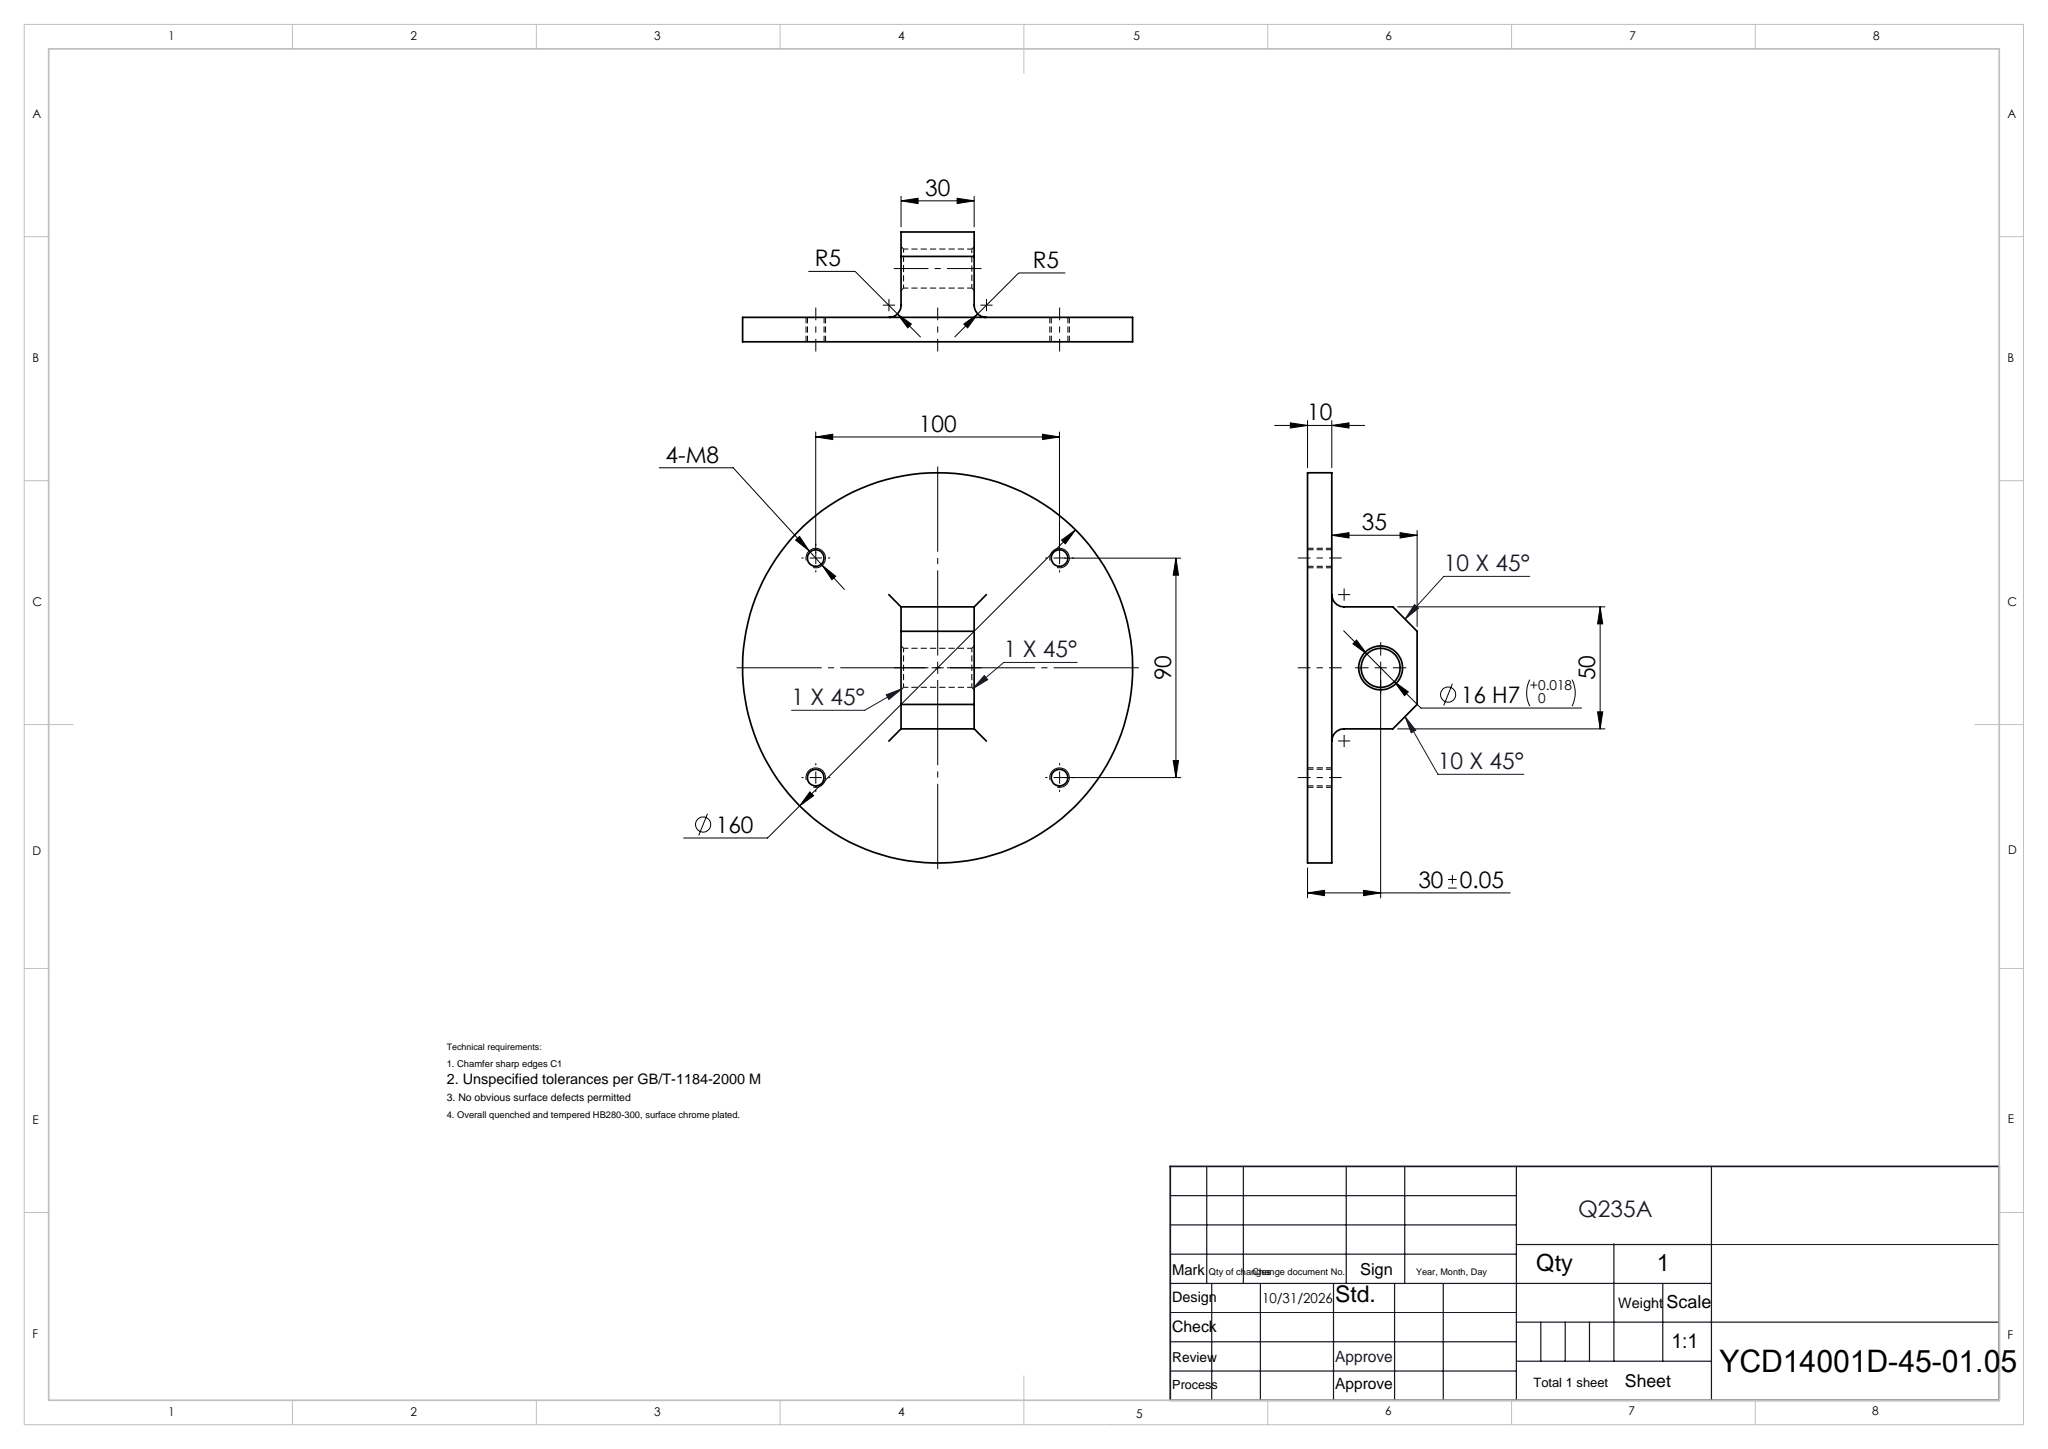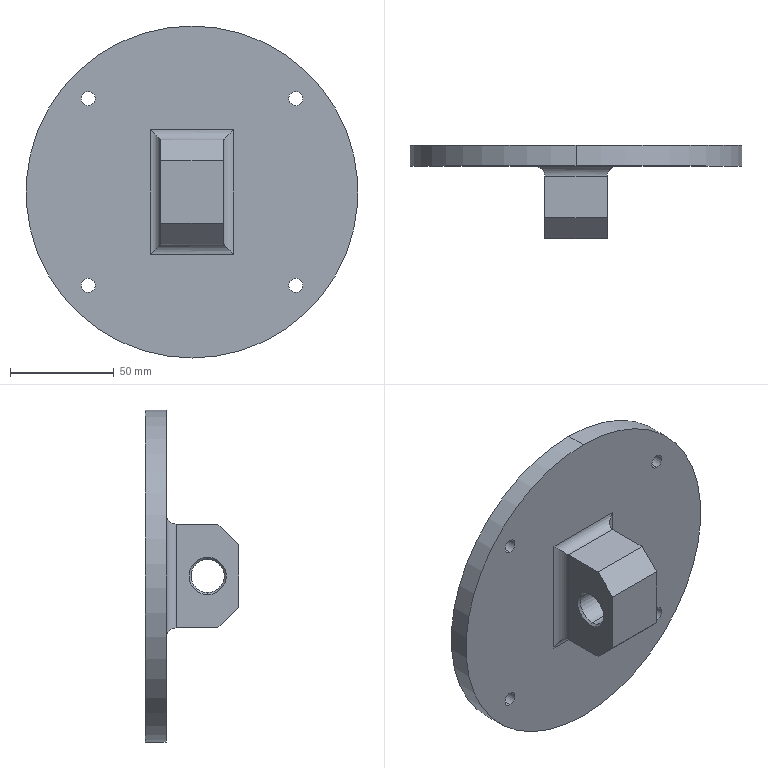Part | SolidWorks | features ICE 3, Chamfer 2, Fillet 2, Extrusion 1, HoleWzd 1 | 1 solid | 29 faces | box 160 x 45 x 160 mm | volume 243931 mm3 | cylinder 16 | plane 9 | cone 4 | commonest cylinder face diameters 6.8 x8 10 x4 16 x2 160 x2
STEP:
#1=CARTESIAN_POINT('',(14.,-25.,8.));
#2=VERTEX_POINT('',#1);
#3=CARTESIAN_POINT('',(14.,-25.,-8.));
#4=VERTEX_POINT('',#3);
#5=CARTESIAN_POINT('',(14.,-25.,0.));
#6=DIRECTION('',(1.,0.,0.));
#7=DIRECTION('',(0.,0.,1.));
#8=AXIS2_PLACEMENT_3D('',#5,#6,#7);
#9=CIRCLE('',#8,8.);
#10=EDGE_CURVE('',#2,#4,#9,.T.);
#11=ORIENTED_EDGE('',*,*,#10,.F.);
#12=CARTESIAN_POINT('',(15.,-25.,9.));
#13=VERTEX_POINT('',#12);
#14=CARTESIAN_POINT('',(14.,-25.,8.));
#15=DIRECTION('',(0.7071,0.,0.7071));
#16=VECTOR('',#15,1000.);
#17=LINE('',#14,#16);
#18=EDGE_CURVE('',#2,#13,#17,.T.);
#19=ORIENTED_EDGE('',*,*,#18,.T.);
#20=CARTESIAN_POINT('',(15.,-25.,-9.));
#21=VERTEX_POINT('',#20);
#22=CARTESIAN_POINT('',(15.,-25.,0.));
#23=DIRECTION('',(-1.,0.,0.));
#24=DIRECTION('',(0.,0.,1.));
#25=AXIS2_PLACEMENT_3D('',#22,#23,#24);
#26=CIRCLE('',#25,9.);
#27=EDGE_CURVE('',#21,#13,#26,.T.);
#28=ORIENTED_EDGE('',*,*,#27,.F.);
#29=CARTESIAN_POINT('',(14.,-25.,-8.));
#30=DIRECTION('',(0.7071,0.,-0.7071));
#31=VECTOR('',#30,1000.);
#32=LINE('',#29,#31);
#33=EDGE_CURVE('',#4,#21,#32,.T.);
#34=ORIENTED_EDGE('',*,*,#33,.F.);
#35=EDGE_LOOP('',(#11,#19,#28,#34));
#36=FACE_OUTER_BOUND('',#35,.T.);
#37=CARTESIAN_POINT('',(14.,-25.,0.));
#38=DIRECTION('',(1.,0.,0.));
#39=DIRECTION('',(0.,0.,-1.));
#40=AXIS2_PLACEMENT_3D('',#37,#38,#39);
#41=CONICAL_SURFACE('',#40,8.,0.7854);
#42=ADVANCED_FACE('',(#36),#41,.F.);
#43=CARTESIAN_POINT('',(-14.,-25.,-8.));
#44=VERTEX_POINT('',#43);
#45=CARTESIAN_POINT('',(-14.,-25.,8.));
#46=VERTEX_POINT('',#45);
#47=CARTESIAN_POINT('',(-14.,-25.,0.));
#48=DIRECTION('',(-1.,0.,0.));
#49=DIRECTION('',(0.,0.,-1.));
#50=AXIS2_PLACEMENT_3D('',#47,#48,#49);
#51=CIRCLE('',#50,8.);
#52=EDGE_CURVE('',#44,#46,#51,.T.);
#53=ORIENTED_EDGE('',*,*,#52,.F.);
#54=CARTESIAN_POINT('',(-15.,-25.,-9.));
#55=VERTEX_POINT('',#54);
#56=CARTESIAN_POINT('',(-15.,-25.,-9.));
#57=DIRECTION('',(-0.7071,0.,-0.7071));
#58=VECTOR('',#57,1000.);
#59=LINE('',#56,#58);
#60=EDGE_CURVE('',#44,#55,#59,.T.);
#61=ORIENTED_EDGE('',*,*,#60,.T.);
#62=CARTESIAN_POINT('',(-15.,-25.,9.));
#63=VERTEX_POINT('',#62);
#64=CARTESIAN_POINT('',(-15.,-25.,0.));
#65=DIRECTION('',(1.,0.,0.));
#66=DIRECTION('',(0.,0.,-1.));
#67=AXIS2_PLACEMENT_3D('',#64,#65,#66);
#68=CIRCLE('',#67,9.);
#69=EDGE_CURVE('',#63,#55,#68,.T.);
#70=ORIENTED_EDGE('',*,*,#69,.F.);
#71=CARTESIAN_POINT('',(-15.,-25.,9.));
#72=DIRECTION('',(-0.7071,0.,0.7071));
#73=VECTOR('',#72,1000.);
#74=LINE('',#71,#73);
#75=EDGE_CURVE('',#46,#63,#74,.T.);
#76=ORIENTED_EDGE('',*,*,#75,.F.);
#77=EDGE_LOOP('',(#53,#61,#70,#76));
#78=FACE_OUTER_BOUND('',#77,.T.);
#79=CARTESIAN_POINT('',(-15.,-25.,0.));
#80=DIRECTION('',(-1.,0.,0.));
#81=DIRECTION('',(0.,0.,1.));
#82=AXIS2_PLACEMENT_3D('',#79,#80,#81);
#83=CONICAL_SURFACE('',#82,9.,0.7854);
#84=ADVANCED_FACE('',(#78),#83,.F.);
#85=ORIENTED_EDGE('',*,*,#52,.T.);
#86=CARTESIAN_POINT('',(-80.,-25.,8.));
#87=DIRECTION('',(1.,0.,0.));
#88=VECTOR('',#87,1000.);
#89=LINE('',#86,#88);
#90=EDGE_CURVE('',#46,#2,#89,.T.);
#91=ORIENTED_EDGE('',*,*,#90,.T.);
#92=ORIENTED_EDGE('',*,*,#10,.T.);
#93=CARTESIAN_POINT('',(-80.,-25.,-8.));
#94=DIRECTION('',(1.,0.,0.));
#95=VECTOR('',#94,1000.);
#96=LINE('',#93,#95);
#97=EDGE_CURVE('',#44,#4,#96,.T.);
#98=ORIENTED_EDGE('',*,*,#97,.F.);
#99=EDGE_LOOP('',(#85,#91,#92,#98));
#100=FACE_OUTER_BOUND('',#99,.T.);
#101=CARTESIAN_POINT('',(-80.,-25.,0.));
#102=DIRECTION('',(1.,0.,0.));
#103=DIRECTION('',(0.,0.,-1.));
#104=AXIS2_PLACEMENT_3D('',#101,#102,#103);
#105=CYLINDRICAL_SURFACE('',#104,8.);
#106=ADVANCED_FACE('',(#100),#105,.F.);
#107=CARTESIAN_POINT('',(-50.,5.,48.4));
#108=VERTEX_POINT('',#107);
#109=CARTESIAN_POINT('',(-50.,5.,41.6));
#110=VERTEX_POINT('',#109);
#111=CARTESIAN_POINT('',(-50.,5.,45.));
#112=DIRECTION('',(0.,-1.,0.));
#113=DIRECTION('',(0.,0.,-1.));
#114=AXIS2_PLACEMENT_3D('',#111,#112,#113);
#115=CIRCLE('',#114,3.4);
#116=EDGE_CURVE('',#108,#110,#115,.T.);
#117=ORIENTED_EDGE('',*,*,#116,.F.);
#118=CARTESIAN_POINT('',(-50.,-5.,48.4));
#119=VERTEX_POINT('',#118);
#120=CARTESIAN_POINT('',(-50.,-5.,48.4));
#121=DIRECTION('',(0.,-1.,0.));
#122=VECTOR('',#121,1000.);
#123=LINE('',#120,#122);
#124=EDGE_CURVE('',#108,#119,#123,.T.);
#125=ORIENTED_EDGE('',*,*,#124,.T.);
#126=CARTESIAN_POINT('',(-50.,-5.,41.6));
#127=VERTEX_POINT('',#126);
#128=CARTESIAN_POINT('',(-50.,-5.,45.));
#129=DIRECTION('',(0.,-1.,0.));
#130=DIRECTION('',(0.,0.,-1.));
#131=AXIS2_PLACEMENT_3D('',#128,#129,#130);
#132=CIRCLE('',#131,3.4);
#133=EDGE_CURVE('',#119,#127,#132,.T.);
#134=ORIENTED_EDGE('',*,*,#133,.T.);
#135=CARTESIAN_POINT('',(-50.,-5.,41.6));
#136=DIRECTION('',(0.,-1.,0.));
#137=VECTOR('',#136,1000.);
#138=LINE('',#135,#137);
#139=EDGE_CURVE('',#110,#127,#138,.T.);
#140=ORIENTED_EDGE('',*,*,#139,.F.);
#141=EDGE_LOOP('',(#117,#125,#134,#140));
#142=FACE_OUTER_BOUND('',#141,.T.);
#143=CARTESIAN_POINT('',(-50.,-5.,45.));
#144=DIRECTION('',(0.,-1.,0.));
#145=DIRECTION('',(0.,0.,-1.));
#146=AXIS2_PLACEMENT_3D('',#143,#144,#145);
#147=CYLINDRICAL_SURFACE('',#146,3.4);
#148=ADVANCED_FACE('',(#142),#147,.F.);
#149=CARTESIAN_POINT('',(-50.,5.,-41.6));
#150=VERTEX_POINT('',#149);
#151=CARTESIAN_POINT('',(-50.,5.,-48.4));
#152=VERTEX_POINT('',#151);
#153=CARTESIAN_POINT('',(-50.,5.,-45.));
#154=DIRECTION('',(0.,-1.,0.));
#155=DIRECTION('',(0.,0.,-1.));
#156=AXIS2_PLACEMENT_3D('',#153,#154,#155);
#157=CIRCLE('',#156,3.4);
#158=EDGE_CURVE('',#150,#152,#157,.T.);
#159=ORIENTED_EDGE('',*,*,#158,.F.);
#160=CARTESIAN_POINT('',(-50.,-5.,-41.6));
#161=VERTEX_POINT('',#160);
#162=CARTESIAN_POINT('',(-50.,-5.,-41.6));
#163=DIRECTION('',(0.,-1.,0.));
#164=VECTOR('',#163,1000.);
#165=LINE('',#162,#164);
#166=EDGE_CURVE('',#150,#161,#165,.T.);
#167=ORIENTED_EDGE('',*,*,#166,.T.);
#168=CARTESIAN_POINT('',(-50.,-5.,-48.4));
#169=VERTEX_POINT('',#168);
#170=CARTESIAN_POINT('',(-50.,-5.,-45.));
#171=DIRECTION('',(0.,-1.,0.));
#172=DIRECTION('',(0.,0.,-1.));
#173=AXIS2_PLACEMENT_3D('',#170,#171,#172);
#174=CIRCLE('',#173,3.4);
#175=EDGE_CURVE('',#161,#169,#174,.T.);
#176=ORIENTED_EDGE('',*,*,#175,.T.);
#177=CARTESIAN_POINT('',(-50.,-5.,-48.4));
#178=DIRECTION('',(0.,-1.,0.));
#179=VECTOR('',#178,1000.);
#180=LINE('',#177,#179);
#181=EDGE_CURVE('',#152,#169,#180,.T.);
#182=ORIENTED_EDGE('',*,*,#181,.F.);
#183=EDGE_LOOP('',(#159,#167,#176,#182));
#184=FACE_OUTER_BOUND('',#183,.T.);
#185=CARTESIAN_POINT('',(-50.,-5.,-45.));
#186=DIRECTION('',(0.,-1.,0.));
#187=DIRECTION('',(0.,0.,-1.));
#188=AXIS2_PLACEMENT_3D('',#185,#186,#187);
#189=CYLINDRICAL_SURFACE('',#188,3.4);
#190=ADVANCED_FACE('',(#184),#189,.F.);
#191=CARTESIAN_POINT('',(50.,5.,-41.6));
#192=VERTEX_POINT('',#191);
#193=CARTESIAN_POINT('',(50.,5.,-48.4));
#194=VERTEX_POINT('',#193);
#195=CARTESIAN_POINT('',(50.,5.,-45.));
#196=DIRECTION('',(0.,-1.,0.));
#197=DIRECTION('',(0.,0.,-1.));
#198=AXIS2_PLACEMENT_3D('',#195,#196,#197);
#199=CIRCLE('',#198,3.4);
#200=EDGE_CURVE('',#192,#194,#199,.T.);
#201=ORIENTED_EDGE('',*,*,#200,.F.);
#202=CARTESIAN_POINT('',(50.,-5.,-41.6));
#203=VERTEX_POINT('',#202);
#204=CARTESIAN_POINT('',(50.,-5.,-41.6));
#205=DIRECTION('',(0.,-1.,0.));
#206=VECTOR('',#205,1000.);
#207=LINE('',#204,#206);
#208=EDGE_CURVE('',#192,#203,#207,.T.);
#209=ORIENTED_EDGE('',*,*,#208,.T.);
#210=CARTESIAN_POINT('',(50.,-5.,-48.4));
#211=VERTEX_POINT('',#210);
#212=CARTESIAN_POINT('',(50.,-5.,-45.));
#213=DIRECTION('',(0.,-1.,0.));
#214=DIRECTION('',(0.,0.,-1.));
#215=AXIS2_PLACEMENT_3D('',#212,#213,#214);
#216=CIRCLE('',#215,3.4);
#217=EDGE_CURVE('',#203,#211,#216,.T.);
#218=ORIENTED_EDGE('',*,*,#217,.T.);
#219=CARTESIAN_POINT('',(50.,-5.,-48.4));
#220=DIRECTION('',(0.,-1.,0.));
#221=VECTOR('',#220,1000.);
#222=LINE('',#219,#221);
#223=EDGE_CURVE('',#194,#211,#222,.T.);
#224=ORIENTED_EDGE('',*,*,#223,.F.);
#225=EDGE_LOOP('',(#201,#209,#218,#224));
#226=FACE_OUTER_BOUND('',#225,.T.);
#227=CARTESIAN_POINT('',(50.,-5.,-45.));
#228=DIRECTION('',(0.,-1.,0.));
#229=DIRECTION('',(0.,0.,-1.));
#230=AXIS2_PLACEMENT_3D('',#227,#228,#229);
#231=CYLINDRICAL_SURFACE('',#230,3.4);
#232=ADVANCED_FACE('',(#226),#231,.F.);
#233=CARTESIAN_POINT('',(50.,5.,48.4));
#234=VERTEX_POINT('',#233);
#235=CARTESIAN_POINT('',(50.,5.,41.6));
#236=VERTEX_POINT('',#235);
#237=CARTESIAN_POINT('',(50.,5.,45.));
#238=DIRECTION('',(0.,-1.,0.));
#239=DIRECTION('',(0.,0.,-1.));
#240=AXIS2_PLACEMENT_3D('',#237,#238,#239);
#241=CIRCLE('',#240,3.4);
#242=EDGE_CURVE('',#234,#236,#241,.T.);
#243=ORIENTED_EDGE('',*,*,#242,.F.);
#244=CARTESIAN_POINT('',(50.,-5.,48.4));
#245=VERTEX_POINT('',#244);
#246=CARTESIAN_POINT('',(50.,-5.,48.4));
#247=DIRECTION('',(0.,-1.,0.));
#248=VECTOR('',#247,1000.);
#249=LINE('',#246,#248);
#250=EDGE_CURVE('',#234,#245,#249,.T.);
#251=ORIENTED_EDGE('',*,*,#250,.T.);
#252=CARTESIAN_POINT('',(50.,-5.,41.6));
#253=VERTEX_POINT('',#252);
#254=CARTESIAN_POINT('',(50.,-5.,45.));
#255=DIRECTION('',(0.,-1.,0.));
#256=DIRECTION('',(0.,0.,-1.));
#257=AXIS2_PLACEMENT_3D('',#254,#255,#256);
#258=CIRCLE('',#257,3.4);
#259=EDGE_CURVE('',#245,#253,#258,.T.);
#260=ORIENTED_EDGE('',*,*,#259,.T.);
#261=CARTESIAN_POINT('',(50.,-5.,41.6));
#262=DIRECTION('',(0.,-1.,0.));
#263=VECTOR('',#262,1000.);
#264=LINE('',#261,#263);
#265=EDGE_CURVE('',#236,#253,#264,.T.);
#266=ORIENTED_EDGE('',*,*,#265,.F.);
#267=EDGE_LOOP('',(#243,#251,#260,#266));
#268=FACE_OUTER_BOUND('',#267,.T.);
#269=CARTESIAN_POINT('',(50.,-5.,45.));
#270=DIRECTION('',(0.,-1.,0.));
#271=DIRECTION('',(0.,0.,-1.));
#272=AXIS2_PLACEMENT_3D('',#269,#270,#271);
#273=CYLINDRICAL_SURFACE('',#272,3.4);
#274=ADVANCED_FACE('',(#268),#273,.F.);
#275=CARTESIAN_POINT('',(0.,5.,80.));
#276=VERTEX_POINT('',#275);
#277=CARTESIAN_POINT('',(0.,5.,-80.));
#278=VERTEX_POINT('',#277);
#279=CARTESIAN_POINT('',(0.,5.,0.));
#280=DIRECTION('',(0.,1.,0.));
#281=DIRECTION('',(0.,0.,1.));
#282=AXIS2_PLACEMENT_3D('',#279,#280,#281);
#283=CIRCLE('',#282,80.);
#284=EDGE_CURVE('',#276,#278,#283,.T.);
#285=ORIENTED_EDGE('',*,*,#284,.F.);
#286=CARTESIAN_POINT('',(0.,-5.,80.));
#287=VERTEX_POINT('',#286);
#288=CARTESIAN_POINT('',(0.,5.,80.));
#289=DIRECTION('',(0.,-1.,0.));
#290=VECTOR('',#289,1000.);
#291=LINE('',#288,#290);
#292=EDGE_CURVE('',#276,#287,#291,.T.);
#293=ORIENTED_EDGE('',*,*,#292,.T.);
#294=CARTESIAN_POINT('',(0.,-5.,-80.));
#295=VERTEX_POINT('',#294);
#296=CARTESIAN_POINT('',(0.,-5.,0.));
#297=DIRECTION('',(0.,1.,0.));
#298=DIRECTION('',(0.,0.,1.));
#299=AXIS2_PLACEMENT_3D('',#296,#297,#298);
#300=CIRCLE('',#299,80.);
#301=EDGE_CURVE('',#287,#295,#300,.T.);
#302=ORIENTED_EDGE('',*,*,#301,.T.);
#303=CARTESIAN_POINT('',(0.,5.,-80.));
#304=DIRECTION('',(0.,-1.,0.));
#305=VECTOR('',#304,1000.);
#306=LINE('',#303,#305);
#307=EDGE_CURVE('',#278,#295,#306,.T.);
#308=ORIENTED_EDGE('',*,*,#307,.F.);
#309=EDGE_LOOP('',(#285,#293,#302,#308));
#310=FACE_OUTER_BOUND('',#309,.T.);
#311=CARTESIAN_POINT('',(0.,5.,0.));
#312=DIRECTION('',(0.,-1.,0.));
#313=DIRECTION('',(0.,0.,-1.));
#314=AXIS2_PLACEMENT_3D('',#311,#312,#313);
#315=CYLINDRICAL_SURFACE('',#314,80.);
#316=ADVANCED_FACE('',(#310),#315,.T.);
#317=CARTESIAN_POINT('',(20.,-5.,30.));
#318=VERTEX_POINT('',#317);
#319=CARTESIAN_POINT('',(20.,-5.,-30.));
#320=VERTEX_POINT('',#319);
#321=CARTESIAN_POINT('',(20.,-5.,-25.));
#322=DIRECTION('',(0.,0.,-1.));
#323=VECTOR('',#322,1000.);
#324=LINE('',#321,#323);
#325=EDGE_CURVE('',#318,#320,#324,.T.);
#326=ORIENTED_EDGE('',*,*,#325,.T.);
#327=CARTESIAN_POINT('',(-20.,-5.,-30.));
#328=VERTEX_POINT('',#327);
#329=CARTESIAN_POINT('',(-15.,-5.,-30.));
#330=DIRECTION('',(-1.,0.,0.));
#331=VECTOR('',#330,1000.);
#332=LINE('',#329,#331);
#333=EDGE_CURVE('',#320,#328,#332,.T.);
#334=ORIENTED_EDGE('',*,*,#333,.T.);
#335=CARTESIAN_POINT('',(-20.,-5.,30.));
#336=VERTEX_POINT('',#335);
#337=CARTESIAN_POINT('',(-20.,-5.,25.));
#338=DIRECTION('',(0.,0.,1.));
#339=VECTOR('',#338,1000.);
#340=LINE('',#337,#339);
#341=EDGE_CURVE('',#328,#336,#340,.T.);
#342=ORIENTED_EDGE('',*,*,#341,.T.);
#343=CARTESIAN_POINT('',(15.,-5.,30.));
#344=DIRECTION('',(1.,0.,0.));
#345=VECTOR('',#344,1000.);
#346=LINE('',#343,#345);
#347=EDGE_CURVE('',#336,#318,#346,.T.);
#348=ORIENTED_EDGE('',*,*,#347,.T.);
#349=EDGE_LOOP('',(#326,#334,#342,#348));
#350=FACE_BOUND('',#349,.T.);
#351=CARTESIAN_POINT('',(0.,-5.,0.));
#352=DIRECTION('',(0.,1.,0.));
#353=DIRECTION('',(0.,0.,1.));
#354=AXIS2_PLACEMENT_3D('',#351,#352,#353);
#355=CIRCLE('',#354,80.);
#356=EDGE_CURVE('',#295,#287,#355,.T.);
#357=ORIENTED_EDGE('',*,*,#356,.F.);
#358=ORIENTED_EDGE('',*,*,#301,.F.);
#359=EDGE_LOOP('',(#357,#358));
#360=FACE_OUTER_BOUND('',#359,.T.);
#361=CARTESIAN_POINT('',(50.,-5.,45.));
#362=DIRECTION('',(0.,-1.,0.));
#363=DIRECTION('',(0.,0.,-1.));
#364=AXIS2_PLACEMENT_3D('',#361,#362,#363);
#365=CIRCLE('',#364,3.4);
#366=EDGE_CURVE('',#253,#245,#365,.T.);
#367=ORIENTED_EDGE('',*,*,#366,.F.);
#368=ORIENTED_EDGE('',*,*,#259,.F.);
#369=EDGE_LOOP('',(#367,#368));
#370=FACE_BOUND('',#369,.T.);
#371=CARTESIAN_POINT('',(50.,-5.,-45.));
#372=DIRECTION('',(0.,-1.,0.));
#373=DIRECTION('',(0.,0.,-1.));
#374=AXIS2_PLACEMENT_3D('',#371,#372,#373);
#375=CIRCLE('',#374,3.4);
#376=EDGE_CURVE('',#211,#203,#375,.T.);
#377=ORIENTED_EDGE('',*,*,#376,.F.);
#378=ORIENTED_EDGE('',*,*,#217,.F.);
#379=EDGE_LOOP('',(#377,#378));
#380=FACE_BOUND('',#379,.T.);
#381=CARTESIAN_POINT('',(-50.,-5.,-45.));
#382=DIRECTION('',(0.,-1.,0.));
#383=DIRECTION('',(0.,0.,-1.));
#384=AXIS2_PLACEMENT_3D('',#381,#382,#383);
#385=CIRCLE('',#384,3.4);
#386=EDGE_CURVE('',#169,#161,#385,.T.);
#387=ORIENTED_EDGE('',*,*,#386,.F.);
#388=ORIENTED_EDGE('',*,*,#175,.F.);
#389=EDGE_LOOP('',(#387,#388));
#390=FACE_BOUND('',#389,.T.);
#391=CARTESIAN_POINT('',(-50.,-5.,45.));
#392=DIRECTION('',(0.,-1.,0.));
#393=DIRECTION('',(0.,0.,-1.));
#394=AXIS2_PLACEMENT_3D('',#391,#392,#393);
#395=CIRCLE('',#394,3.4);
#396=EDGE_CURVE('',#127,#119,#395,.T.);
#397=ORIENTED_EDGE('',*,*,#396,.F.);
#398=ORIENTED_EDGE('',*,*,#133,.F.);
#399=EDGE_LOOP('',(#397,#398));
#400=FACE_BOUND('',#399,.T.);
#401=CARTESIAN_POINT('',(0.,-5.,0.));
#402=DIRECTION('',(0.,1.,0.));
#403=DIRECTION('',(0.,0.,1.));
#404=AXIS2_PLACEMENT_3D('',#401,#402,#403);
#405=PLANE('',#404);
#406=ADVANCED_FACE('',(#350,#360,#370,#380,#390,#400),#405,.F.);
#407=ORIENTED_EDGE('',*,*,#292,.F.);
#408=CARTESIAN_POINT('',(0.,5.,0.));
#409=DIRECTION('',(0.,1.,0.));
#410=DIRECTION('',(0.,0.,1.));
#411=AXIS2_PLACEMENT_3D('',#408,#409,#410);
#412=CIRCLE('',#411,80.);
#413=EDGE_CURVE('',#278,#276,#412,.T.);
#414=ORIENTED_EDGE('',*,*,#413,.F.);
#415=ORIENTED_EDGE('',*,*,#307,.T.);
#416=ORIENTED_EDGE('',*,*,#356,.T.);
#417=EDGE_LOOP('',(#407,#414,#415,#416));
#418=FACE_OUTER_BOUND('',#417,.T.);
#419=CARTESIAN_POINT('',(0.,5.,0.));
#420=DIRECTION('',(0.,-1.,0.));
#421=DIRECTION('',(0.,0.,-1.));
#422=AXIS2_PLACEMENT_3D('',#419,#420,#421);
#423=CYLINDRICAL_SURFACE('',#422,80.);
#424=ADVANCED_FACE('',(#418),#423,.T.);
#425=CARTESIAN_POINT('',(-50.,5.,45.));
#426=DIRECTION('',(0.,-1.,0.));
#427=DIRECTION('',(0.,0.,-1.));
#428=AXIS2_PLACEMENT_3D('',#425,#426,#427);
#429=CIRCLE('',#428,3.4);
#430=EDGE_CURVE('',#110,#108,#429,.T.);
#431=ORIENTED_EDGE('',*,*,#430,.T.);
#432=ORIENTED_EDGE('',*,*,#116,.T.);
#433=EDGE_LOOP('',(#431,#432));
#434=FACE_BOUND('',#433,.T.);
#435=CARTESIAN_POINT('',(-50.,5.,-45.));
#436=DIRECTION('',(0.,-1.,0.));
#437=DIRECTION('',(0.,0.,-1.));
#438=AXIS2_PLACEMENT_3D('',#435,#436,#437);
#439=CIRCLE('',#438,3.4);
#440=EDGE_CURVE('',#152,#150,#439,.T.);
#441=ORIENTED_EDGE('',*,*,#440,.T.);
#442=ORIENTED_EDGE('',*,*,#158,.T.);
#443=EDGE_LOOP('',(#441,#442));
#444=FACE_BOUND('',#443,.T.);
#445=CARTESIAN_POINT('',(50.,5.,-45.));
#446=DIRECTION('',(0.,-1.,0.));
#447=DIRECTION('',(0.,0.,-1.));
#448=AXIS2_PLACEMENT_3D('',#445,#446,#447);
#449=CIRCLE('',#448,3.4);
#450=EDGE_CURVE('',#194,#192,#449,.T.);
#451=ORIENTED_EDGE('',*,*,#450,.T.);
#452=ORIENTED_EDGE('',*,*,#200,.T.);
#453=EDGE_LOOP('',(#451,#452));
#454=FACE_BOUND('',#453,.T.);
#455=CARTESIAN_POINT('',(50.,5.,45.));
#456=DIRECTION('',(0.,-1.,0.));
#457=DIRECTION('',(0.,0.,-1.));
#458=AXIS2_PLACEMENT_3D('',#455,#456,#457);
#459=CIRCLE('',#458,3.4);
#460=EDGE_CURVE('',#236,#234,#459,.T.);
#461=ORIENTED_EDGE('',*,*,#460,.T.);
#462=ORIENTED_EDGE('',*,*,#242,.T.);
#463=EDGE_LOOP('',(#461,#462));
#464=FACE_BOUND('',#463,.T.);
#465=ORIENTED_EDGE('',*,*,#413,.T.);
#466=ORIENTED_EDGE('',*,*,#284,.T.);
#467=EDGE_LOOP('',(#465,#466));
#468=FACE_OUTER_BOUND('',#467,.T.);
#469=CARTESIAN_POINT('',(0.,5.,0.));
#470=DIRECTION('',(0.,1.,0.));
#471=DIRECTION('',(0.,0.,1.));
#472=AXIS2_PLACEMENT_3D('',#469,#470,#471);
#473=PLANE('',#472);
#474=ADVANCED_FACE('',(#434,#444,#454,#464,#468),#473,.T.);
#475=ORIENTED_EDGE('',*,*,#250,.F.);
#476=ORIENTED_EDGE('',*,*,#460,.F.);
#477=ORIENTED_EDGE('',*,*,#265,.T.);
#478=ORIENTED_EDGE('',*,*,#366,.T.);
#479=EDGE_LOOP('',(#475,#476,#477,#478));
#480=FACE_OUTER_BOUND('',#479,.T.);
#481=CARTESIAN_POINT('',(50.,-5.,45.));
#482=DIRECTION('',(0.,-1.,0.));
#483=DIRECTION('',(0.,0.,-1.));
#484=AXIS2_PLACEMENT_3D('',#481,#482,#483);
#485=CYLINDRICAL_SURFACE('',#484,3.4);
#486=ADVANCED_FACE('',(#480),#485,.F.);
#487=ORIENTED_EDGE('',*,*,#208,.F.);
#488=ORIENTED_EDGE('',*,*,#450,.F.);
#489=ORIENTED_EDGE('',*,*,#223,.T.);
#490=ORIENTED_EDGE('',*,*,#376,.T.);
#491=EDGE_LOOP('',(#487,#488,#489,#490));
#492=FACE_OUTER_BOUND('',#491,.T.);
#493=CARTESIAN_POINT('',(50.,-5.,-45.));
#494=DIRECTION('',(0.,-1.,0.));
#495=DIRECTION('',(0.,0.,-1.));
#496=AXIS2_PLACEMENT_3D('',#493,#494,#495);
#497=CYLINDRICAL_SURFACE('',#496,3.4);
#498=ADVANCED_FACE('',(#492),#497,.F.);
#499=ORIENTED_EDGE('',*,*,#166,.F.);
#500=ORIENTED_EDGE('',*,*,#440,.F.);
#501=ORIENTED_EDGE('',*,*,#181,.T.);
#502=ORIENTED_EDGE('',*,*,#386,.T.);
#503=EDGE_LOOP('',(#499,#500,#501,#502));
#504=FACE_OUTER_BOUND('',#503,.T.);
#505=CARTESIAN_POINT('',(-50.,-5.,-45.));
#506=DIRECTION('',(0.,-1.,0.));
#507=DIRECTION('',(0.,0.,-1.));
#508=AXIS2_PLACEMENT_3D('',#505,#506,#507);
#509=CYLINDRICAL_SURFACE('',#508,3.4);
#510=ADVANCED_FACE('',(#504),#509,.F.);
#511=ORIENTED_EDGE('',*,*,#124,.F.);
#512=ORIENTED_EDGE('',*,*,#430,.F.);
#513=ORIENTED_EDGE('',*,*,#139,.T.);
#514=ORIENTED_EDGE('',*,*,#396,.T.);
#515=EDGE_LOOP('',(#511,#512,#513,#514));
#516=FACE_OUTER_BOUND('',#515,.T.);
#517=CARTESIAN_POINT('',(-50.,-5.,45.));
#518=DIRECTION('',(0.,-1.,0.));
#519=DIRECTION('',(0.,0.,-1.));
#520=AXIS2_PLACEMENT_3D('',#517,#518,#519);
#521=CYLINDRICAL_SURFACE('',#520,3.4);
#522=ADVANCED_FACE('',(#516),#521,.F.);
#523=ORIENTED_EDGE('',*,*,#27,.T.);
#524=CARTESIAN_POINT('',(15.,-25.,0.));
#525=DIRECTION('',(-1.,0.,0.));
#526=DIRECTION('',(0.,0.,1.));
#527=AXIS2_PLACEMENT_3D('',#524,#525,#526);
#528=CIRCLE('',#527,9.);
#529=EDGE_CURVE('',#13,#21,#528,.T.);
#530=ORIENTED_EDGE('',*,*,#529,.T.);
#531=EDGE_LOOP('',(#523,#530));
#532=FACE_BOUND('',#531,.T.);
#533=CARTESIAN_POINT('',(15.,-30.,-25.));
#534=VERTEX_POINT('',#533);
#535=CARTESIAN_POINT('',(15.,-10.,-25.));
#536=VERTEX_POINT('',#535);
#537=CARTESIAN_POINT('',(15.,-40.,-25.));
#538=DIRECTION('',(0.,1.,0.));
#539=VECTOR('',#538,1000.);
#540=LINE('',#537,#539);
#541=EDGE_CURVE('',#534,#536,#540,.T.);
#542=ORIENTED_EDGE('',*,*,#541,.T.);
#543=CARTESIAN_POINT('',(15.,-10.,25.));
#544=VERTEX_POINT('',#543);
#545=CARTESIAN_POINT('',(15.,-10.,25.));
#546=DIRECTION('',(0.,0.,1.));
#547=VECTOR('',#546,1000.);
#548=LINE('',#545,#547);
#549=EDGE_CURVE('',#536,#544,#548,.T.);
#550=ORIENTED_EDGE('',*,*,#549,.T.);
#551=CARTESIAN_POINT('',(15.,-30.,25.));
#552=VERTEX_POINT('',#551);
#553=CARTESIAN_POINT('',(15.,-40.,25.));
#554=DIRECTION('',(0.,1.,0.));
#555=VECTOR('',#554,1000.);
#556=LINE('',#553,#555);
#557=EDGE_CURVE('',#552,#544,#556,.T.);
#558=ORIENTED_EDGE('',*,*,#557,.F.);
#559=CARTESIAN_POINT('',(15.,-40.,15.));
#560=VERTEX_POINT('',#559);
#561=CARTESIAN_POINT('',(15.,-40.,15.));
#562=DIRECTION('',(0.,-0.7071,-0.7071));
#563=VECTOR('',#562,1000.);
#564=LINE('',#561,#563);
#565=EDGE_CURVE('',#552,#560,#564,.T.);
#566=ORIENTED_EDGE('',*,*,#565,.T.);
#567=CARTESIAN_POINT('',(15.,-40.,-15.));
#568=VERTEX_POINT('',#567);
#569=CARTESIAN_POINT('',(15.,-40.,25.));
#570=DIRECTION('',(0.,0.,1.));
#571=VECTOR('',#570,1000.);
#572=LINE('',#569,#571);
#573=EDGE_CURVE('',#568,#560,#572,.T.);
#574=ORIENTED_EDGE('',*,*,#573,.F.);
#575=CARTESIAN_POINT('',(15.,-40.,-15.));
#576=DIRECTION('',(0.,0.7071,-0.7071));
#577=VECTOR('',#576,1000.);
#578=LINE('',#575,#577);
#579=EDGE_CURVE('',#568,#534,#578,.T.);
#580=ORIENTED_EDGE('',*,*,#579,.T.);
#581=EDGE_LOOP('',(#542,#550,#558,#566,#574,#580));
#582=FACE_OUTER_BOUND('',#581,.T.);
#583=CARTESIAN_POINT('',(15.,-40.,25.));
#584=DIRECTION('',(-1.,0.,0.));
#585=DIRECTION('',(0.,0.,1.));
#586=AXIS2_PLACEMENT_3D('',#583,#584,#585);
#587=PLANE('',#586);
#588=ADVANCED_FACE('',(#532,#582),#587,.F.);
#589=ORIENTED_EDGE('',*,*,#557,.T.);
#590=CARTESIAN_POINT('',(-15.,-10.,25.));
#591=VERTEX_POINT('',#590);
#592=CARTESIAN_POINT('',(-15.,-10.,25.));
#593=DIRECTION('',(-1.,0.,0.));
#594=VECTOR('',#593,1000.);
#595=LINE('',#592,#594);
#596=EDGE_CURVE('',#544,#591,#595,.T.);
#597=ORIENTED_EDGE('',*,*,#596,.T.);
#598=CARTESIAN_POINT('',(-15.,-30.,25.));
#599=VERTEX_POINT('',#598);
#600=CARTESIAN_POINT('',(-15.,-40.,25.));
#601=DIRECTION('',(0.,1.,0.));
#602=VECTOR('',#601,1000.);
#603=LINE('',#600,#602);
#604=EDGE_CURVE('',#599,#591,#603,.T.);
#605=ORIENTED_EDGE('',*,*,#604,.F.);
#606=CARTESIAN_POINT('',(15.,-30.,25.));
#607=DIRECTION('',(1.,0.,0.));
#608=VECTOR('',#607,1000.);
#609=LINE('',#606,#608);
#610=EDGE_CURVE('',#599,#552,#609,.T.);
#611=ORIENTED_EDGE('',*,*,#610,.T.);
#612=EDGE_LOOP('',(#589,#597,#605,#611));
#613=FACE_OUTER_BOUND('',#612,.T.);
#614=CARTESIAN_POINT('',(-15.,-40.,25.));
#615=DIRECTION('',(0.,0.,-1.));
#616=DIRECTION('',(0.,1.,0.));
#617=AXIS2_PLACEMENT_3D('',#614,#615,#616);
#618=PLANE('',#617);
#619=ADVANCED_FACE('',(#613),#618,.F.);
#620=ORIENTED_EDGE('',*,*,#69,.T.);
#621=CARTESIAN_POINT('',(-15.,-25.,0.));
#622=DIRECTION('',(1.,0.,0.));
#623=DIRECTION('',(0.,0.,-1.));
#624=AXIS2_PLACEMENT_3D('',#621,#622,#623);
#625=CIRCLE('',#624,9.);
#626=EDGE_CURVE('',#55,#63,#625,.T.);
#627=ORIENTED_EDGE('',*,*,#626,.T.);
#628=EDGE_LOOP('',(#620,#627));
#629=FACE_BOUND('',#628,.T.);
#630=ORIENTED_EDGE('',*,*,#604,.T.);
#631=CARTESIAN_POINT('',(-15.,-10.,-25.));
#632=VERTEX_POINT('',#631);
#633=CARTESIAN_POINT('',(-15.,-10.,-25.));
#634=DIRECTION('',(0.,0.,-1.));
#635=VECTOR('',#634,1000.);
#636=LINE('',#633,#635);
#637=EDGE_CURVE('',#591,#632,#636,.T.);
#638=ORIENTED_EDGE('',*,*,#637,.T.);
#639=CARTESIAN_POINT('',(-15.,-30.,-25.));
#640=VERTEX_POINT('',#639);
#641=CARTESIAN_POINT('',(-15.,-40.,-25.));
#642=DIRECTION('',(0.,1.,0.));
#643=VECTOR('',#642,1000.);
#644=LINE('',#641,#643);
#645=EDGE_CURVE('',#640,#632,#644,.T.);
#646=ORIENTED_EDGE('',*,*,#645,.F.);
#647=CARTESIAN_POINT('',(-15.,-40.,-15.));
#648=VERTEX_POINT('',#647);
#649=CARTESIAN_POINT('',(-15.,-40.,-15.));
#650=DIRECTION('',(0.,-0.7071,0.7071));
#651=VECTOR('',#650,1000.);
#652=LINE('',#649,#651);
#653=EDGE_CURVE('',#640,#648,#652,.T.);
#654=ORIENTED_EDGE('',*,*,#653,.T.);
#655=CARTESIAN_POINT('',(-15.,-40.,15.));
#656=VERTEX_POINT('',#655);
#657=CARTESIAN_POINT('',(-15.,-40.,25.));
#658=DIRECTION('',(0.,0.,-1.));
#659=VECTOR('',#658,1000.);
#660=LINE('',#657,#659);
#661=EDGE_CURVE('',#656,#648,#660,.T.);
#662=ORIENTED_EDGE('',*,*,#661,.F.);
#663=CARTESIAN_POINT('',(-15.,-40.,15.));
#664=DIRECTION('',(0.,0.7071,0.7071));
#665=VECTOR('',#664,1000.);
#666=LINE('',#663,#665);
#667=EDGE_CURVE('',#656,#599,#666,.T.);
#668=ORIENTED_EDGE('',*,*,#667,.T.);
#669=EDGE_LOOP('',(#630,#638,#646,#654,#662,#668));
#670=FACE_OUTER_BOUND('',#669,.T.);
#671=CARTESIAN_POINT('',(-15.,-40.,25.));
#672=DIRECTION('',(1.,0.,0.));
#673=DIRECTION('',(0.,0.,-1.));
#674=AXIS2_PLACEMENT_3D('',#671,#672,#673);
#675=PLANE('',#674);
#676=ADVANCED_FACE('',(#629,#670),#675,.F.);
#677=ORIENTED_EDGE('',*,*,#645,.T.);
#678=CARTESIAN_POINT('',(15.,-10.,-25.));
#679=DIRECTION('',(1.,0.,0.));
#680=VECTOR('',#679,1000.);
#681=LINE('',#678,#680);
#682=EDGE_CURVE('',#632,#536,#681,.T.);
#683=ORIENTED_EDGE('',*,*,#682,.T.);
#684=ORIENTED_EDGE('',*,*,#541,.F.);
#685=CARTESIAN_POINT('',(-15.,-30.,-25.));
#686=DIRECTION('',(-1.,0.,0.));
#687=VECTOR('',#686,1000.);
#688=LINE('',#685,#687);
#689=EDGE_CURVE('',#534,#640,#688,.T.);
#690=ORIENTED_EDGE('',*,*,#689,.T.);
#691=EDGE_LOOP('',(#677,#683,#684,#690));
#692=FACE_OUTER_BOUND('',#691,.T.);
#693=CARTESIAN_POINT('',(-15.,-40.,-25.));
#694=DIRECTION('',(0.,0.,1.));
#695=DIRECTION('',(0.,-1.,0.));
#696=AXIS2_PLACEMENT_3D('',#693,#694,#695);
#697=PLANE('',#696);
#698=ADVANCED_FACE('',(#692),#697,.F.);
#699=ORIENTED_EDGE('',*,*,#661,.T.);
#700=CARTESIAN_POINT('',(15.,-40.,-15.));
#701=DIRECTION('',(1.,0.,0.));
#702=VECTOR('',#701,1000.);
#703=LINE('',#700,#702);
#704=EDGE_CURVE('',#648,#568,#703,.T.);
#705=ORIENTED_EDGE('',*,*,#704,.T.);
#706=ORIENTED_EDGE('',*,*,#573,.T.);
#707=CARTESIAN_POINT('',(-15.,-40.,15.));
#708=DIRECTION('',(-1.,0.,0.));
#709=VECTOR('',#708,1000.);
#710=LINE('',#707,#709);
#711=EDGE_CURVE('',#560,#656,#710,.T.);
#712=ORIENTED_EDGE('',*,*,#711,.T.);
#713=EDGE_LOOP('',(#699,#705,#706,#712));
#714=FACE_OUTER_BOUND('',#713,.T.);
#715=CARTESIAN_POINT('',(0.,-40.,0.));
#716=DIRECTION('',(0.,-1.,0.));
#717=DIRECTION('',(0.,0.,-1.));
#718=AXIS2_PLACEMENT_3D('',#715,#716,#717);
#719=PLANE('',#718);
#720=ADVANCED_FACE('',(#714),#719,.T.);
#721=ORIENTED_EDGE('',*,*,#90,.F.);
#722=CARTESIAN_POINT('',(-14.,-25.,0.));
#723=DIRECTION('',(-1.,0.,0.));
#724=DIRECTION('',(0.,0.,-1.));
#725=AXIS2_PLACEMENT_3D('',#722,#723,#724);
#726=CIRCLE('',#725,8.);
#727=EDGE_CURVE('',#46,#44,#726,.T.);
#728=ORIENTED_EDGE('',*,*,#727,.T.);
#729=ORIENTED_EDGE('',*,*,#97,.T.);
#730=CARTESIAN_POINT('',(14.,-25.,0.));
#731=DIRECTION('',(1.,0.,0.));
#732=DIRECTION('',(0.,0.,1.));
#733=AXIS2_PLACEMENT_3D('',#730,#731,#732);
#734=CIRCLE('',#733,8.);
#735=EDGE_CURVE('',#4,#2,#734,.T.);
#736=ORIENTED_EDGE('',*,*,#735,.T.);
#737=EDGE_LOOP('',(#721,#728,#729,#736));
#738=FACE_OUTER_BOUND('',#737,.T.);
#739=CARTESIAN_POINT('',(-80.,-25.,0.));
#740=DIRECTION('',(1.,0.,0.));
#741=DIRECTION('',(0.,0.,-1.));
#742=AXIS2_PLACEMENT_3D('',#739,#740,#741);
#743=CYLINDRICAL_SURFACE('',#742,8.);
#744=ADVANCED_FACE('',(#738),#743,.F.);
#745=ORIENTED_EDGE('',*,*,#653,.F.);
#746=ORIENTED_EDGE('',*,*,#689,.F.);
#747=ORIENTED_EDGE('',*,*,#579,.F.);
#748=ORIENTED_EDGE('',*,*,#704,.F.);
#749=EDGE_LOOP('',(#745,#746,#747,#748));
#750=FACE_OUTER_BOUND('',#749,.T.);
#751=CARTESIAN_POINT('',(0.,-40.,-15.));
#752=DIRECTION('',(0.,-0.7071,-0.7071));
#753=DIRECTION('',(-1.,0.,0.));
#754=AXIS2_PLACEMENT_3D('',#751,#752,#753);
#755=PLANE('',#754);
#756=ADVANCED_FACE('',(#750),#755,.T.);
#757=ORIENTED_EDGE('',*,*,#565,.F.);
#758=ORIENTED_EDGE('',*,*,#610,.F.);
#759=ORIENTED_EDGE('',*,*,#667,.F.);
#760=ORIENTED_EDGE('',*,*,#711,.F.);
#761=EDGE_LOOP('',(#757,#758,#759,#760));
#762=FACE_OUTER_BOUND('',#761,.T.);
#763=CARTESIAN_POINT('',(0.,-40.,15.));
#764=DIRECTION('',(0.,-0.7071,0.7071));
#765=DIRECTION('',(1.,0.,0.));
#766=AXIS2_PLACEMENT_3D('',#763,#764,#765);
#767=PLANE('',#766);
#768=ADVANCED_FACE('',(#762),#767,.T.);
#769=CARTESIAN_POINT('',(20.,-5.,30.));
#770=CARTESIAN_POINT('',(17.071,-5.,27.071));
#771=CARTESIAN_POINT('',(15.,-7.071,25.));
#772=CARTESIAN_POINT('',(15.,-10.,25.));
#773=(BOUNDED_CURVE()B_SPLINE_CURVE(3,(#769,#770,#771,#772),.UNSPECIFIED.,.F.,.F.)B_SPLINE_CURVE_WITH_KNOTS((4,4),(1.571,3.142),.UNSPECIFIED.)CURVE()GEOMETRIC_REPRESENTATION_ITEM()RATIONAL_B_SPLINE_CURVE((1.,0.8047,0.8047,1.))REPRESENTATION_ITEM(''));
#774=EDGE_CURVE('',#318,#544,#773,.T.);
#775=ORIENTED_EDGE('',*,*,#774,.F.);
#776=ORIENTED_EDGE('',*,*,#347,.F.);
#777=CARTESIAN_POINT('',(-15.,-10.,25.));
#778=CARTESIAN_POINT('',(-15.,-7.071,25.));
#779=CARTESIAN_POINT('',(-17.071,-5.,27.071));
#780=CARTESIAN_POINT('',(-20.,-5.,30.));
#781=(BOUNDED_CURVE()B_SPLINE_CURVE(3,(#777,#778,#779,#780),.UNSPECIFIED.,.F.,.F.)B_SPLINE_CURVE_WITH_KNOTS((4,4),(3.142,4.712),.UNSPECIFIED.)CURVE()GEOMETRIC_REPRESENTATION_ITEM()RATIONAL_B_SPLINE_CURVE((1.,0.8047,0.8047,1.))REPRESENTATION_ITEM(''));
#782=EDGE_CURVE('',#591,#336,#781,.T.);
#783=ORIENTED_EDGE('',*,*,#782,.F.);
#784=ORIENTED_EDGE('',*,*,#596,.F.);
#785=EDGE_LOOP('',(#775,#776,#783,#784));
#786=FACE_OUTER_BOUND('',#785,.T.);
#787=CARTESIAN_POINT('',(-15.,-10.,30.));
#788=DIRECTION('',(1.,0.,0.));
#789=DIRECTION('',(0.,0.,-1.));
#790=AXIS2_PLACEMENT_3D('',#787,#788,#789);
#791=CYLINDRICAL_SURFACE('',#790,5.);
#792=ADVANCED_FACE('',(#786),#791,.F.);
#793=ORIENTED_EDGE('',*,*,#782,.T.);
#794=ORIENTED_EDGE('',*,*,#341,.F.);
#795=CARTESIAN_POINT('',(-15.,-10.,-25.));
#796=CARTESIAN_POINT('',(-15.,-7.071,-25.));
#797=CARTESIAN_POINT('',(-17.071,-5.,-27.071));
#798=CARTESIAN_POINT('',(-20.,-5.,-30.));
#799=(BOUNDED_CURVE()B_SPLINE_CURVE(3,(#795,#796,#797,#798),.UNSPECIFIED.,.F.,.F.)B_SPLINE_CURVE_WITH_KNOTS((4,4),(0.,1.571),.UNSPECIFIED.)CURVE()GEOMETRIC_REPRESENTATION_ITEM()RATIONAL_B_SPLINE_CURVE((1.,0.8047,0.8047,1.))REPRESENTATION_ITEM(''));
#800=EDGE_CURVE('',#632,#328,#799,.T.);
#801=ORIENTED_EDGE('',*,*,#800,.F.);
#802=ORIENTED_EDGE('',*,*,#637,.F.);
#803=EDGE_LOOP('',(#793,#794,#801,#802));
#804=FACE_OUTER_BOUND('',#803,.T.);
#805=CARTESIAN_POINT('',(-20.,-10.,25.));
#806=DIRECTION('',(0.,0.,1.));
#807=DIRECTION('',(1.,0.,0.));
#808=AXIS2_PLACEMENT_3D('',#805,#806,#807);
#809=CYLINDRICAL_SURFACE('',#808,5.);
#810=ADVANCED_FACE('',(#804),#809,.F.);
#811=ORIENTED_EDGE('',*,*,#774,.T.);
#812=ORIENTED_EDGE('',*,*,#549,.F.);
#813=CARTESIAN_POINT('',(20.,-5.,-30.));
#814=CARTESIAN_POINT('',(17.071,-5.,-27.071));
#815=CARTESIAN_POINT('',(15.,-7.071,-25.));
#816=CARTESIAN_POINT('',(15.,-10.,-25.));
#817=(BOUNDED_CURVE()B_SPLINE_CURVE(3,(#813,#814,#815,#816),.UNSPECIFIED.,.F.,.F.)B_SPLINE_CURVE_WITH_KNOTS((4,4),(1.571,3.142),.UNSPECIFIED.)CURVE()GEOMETRIC_REPRESENTATION_ITEM()RATIONAL_B_SPLINE_CURVE((1.,0.8047,0.8047,1.))REPRESENTATION_ITEM(''));
#818=EDGE_CURVE('',#320,#536,#817,.T.);
#819=ORIENTED_EDGE('',*,*,#818,.F.);
#820=ORIENTED_EDGE('',*,*,#325,.F.);
#821=EDGE_LOOP('',(#811,#812,#819,#820));
#822=FACE_OUTER_BOUND('',#821,.T.);
#823=CARTESIAN_POINT('',(20.,-10.,25.));
#824=DIRECTION('',(0.,0.,-1.));
#825=DIRECTION('',(-1.,0.,0.));
#826=AXIS2_PLACEMENT_3D('',#823,#824,#825);
#827=CYLINDRICAL_SURFACE('',#826,5.);
#828=ADVANCED_FACE('',(#822),#827,.F.);
#829=ORIENTED_EDGE('',*,*,#800,.T.);
#830=ORIENTED_EDGE('',*,*,#333,.F.);
#831=ORIENTED_EDGE('',*,*,#818,.T.);
#832=ORIENTED_EDGE('',*,*,#682,.F.);
#833=EDGE_LOOP('',(#829,#830,#831,#832));
#834=FACE_OUTER_BOUND('',#833,.T.);
#835=CARTESIAN_POINT('',(-15.,-10.,-30.));
#836=DIRECTION('',(-1.,0.,0.));
#837=DIRECTION('',(0.,0.,1.));
#838=AXIS2_PLACEMENT_3D('',#835,#836,#837);
#839=CYLINDRICAL_SURFACE('',#838,5.);
#840=ADVANCED_FACE('',(#834),#839,.F.);
#841=ORIENTED_EDGE('',*,*,#60,.F.);
#842=ORIENTED_EDGE('',*,*,#727,.F.);
#843=ORIENTED_EDGE('',*,*,#75,.T.);
#844=ORIENTED_EDGE('',*,*,#626,.F.);
#845=EDGE_LOOP('',(#841,#842,#843,#844));
#846=FACE_OUTER_BOUND('',#845,.T.);
#847=CARTESIAN_POINT('',(-15.,-25.,0.));
#848=DIRECTION('',(-1.,0.,0.));
#849=DIRECTION('',(0.,0.,1.));
#850=AXIS2_PLACEMENT_3D('',#847,#848,#849);
#851=CONICAL_SURFACE('',#850,9.,0.7854);
#852=ADVANCED_FACE('',(#846),#851,.F.);
#853=ORIENTED_EDGE('',*,*,#18,.F.);
#854=ORIENTED_EDGE('',*,*,#735,.F.);
#855=ORIENTED_EDGE('',*,*,#33,.T.);
#856=ORIENTED_EDGE('',*,*,#529,.F.);
#857=EDGE_LOOP('',(#853,#854,#855,#856));
#858=FACE_OUTER_BOUND('',#857,.T.);
#859=CARTESIAN_POINT('',(14.,-25.,0.));
#860=DIRECTION('',(1.,0.,0.));
#861=DIRECTION('',(0.,0.,-1.));
#862=AXIS2_PLACEMENT_3D('',#859,#860,#861);
#863=CONICAL_SURFACE('',#862,8.,0.7854);
#864=ADVANCED_FACE('',(#858),#863,.F.);
#865=CLOSED_SHELL('',(#42,#84,#106,#148,#190,#232,#274,#316,#406,#424,#474,#486,#498,#510,#522,#588,#619,#676,#698,#720,#744,#756,#768,#792,#810,#828,#840,#852,#864));
#866=MANIFOLD_SOLID_BREP('',#865);
#867=CARTESIAN_POINT('',(0.,0.,0.));
#868=DIRECTION('',(0.,0.,1.));
#869=DIRECTION('',(1.,0.,0.));
#870=AXIS2_PLACEMENT_3D('',#867,#868,#869);
#871=(LENGTH_UNIT()NAMED_UNIT(*)SI_UNIT(.MILLI.,.METRE.));
#872=UNCERTAINTY_MEASURE_WITH_UNIT(LENGTH_MEASURE(0.00001),#871,'','');
#873=(NAMED_UNIT(*)PLANE_ANGLE_UNIT()SI_UNIT($,.RADIAN.));
#874=(NAMED_UNIT(*)SI_UNIT($,.STERADIAN.)SOLID_ANGLE_UNIT());
#875=(GEOMETRIC_REPRESENTATION_CONTEXT(3)GLOBAL_UNCERTAINTY_ASSIGNED_CONTEXT((#872))GLOBAL_UNIT_ASSIGNED_CONTEXT((#871,#873,#874))REPRESENTATION_CONTEXT('',''));
#876=ADVANCED_BREP_SHAPE_REPRESENTATION('',(#866,#870),#875);